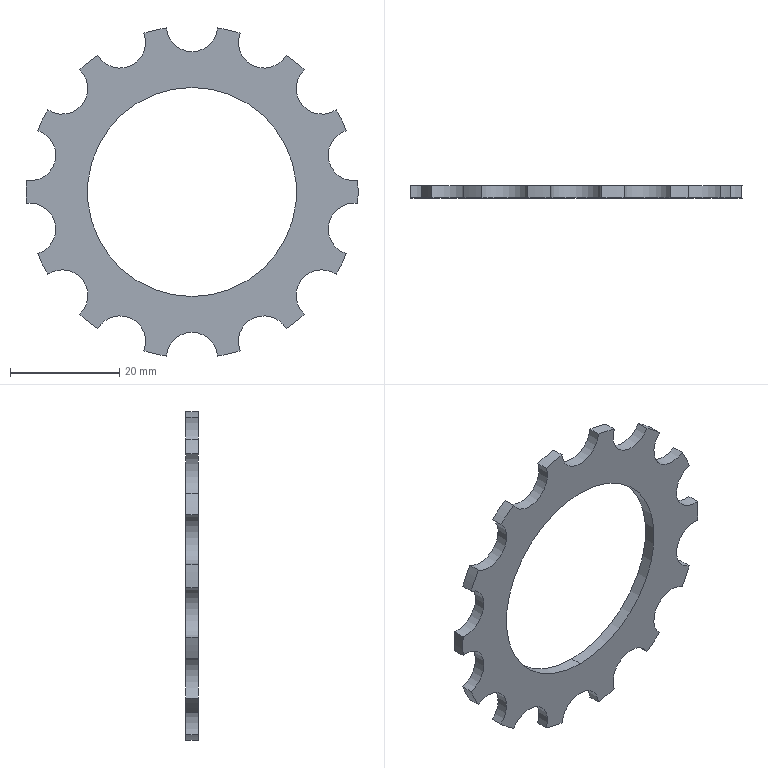Part | STEP file | Gear 5 | 1 solid | 39 faces | box 60.7 x 2.2 x 59.972 mm | volume 2811 mm3 | cylinder 37 | plane 2 | commonest cylinder face diameters 9.4 x21 60.7 x14 38.2 x2